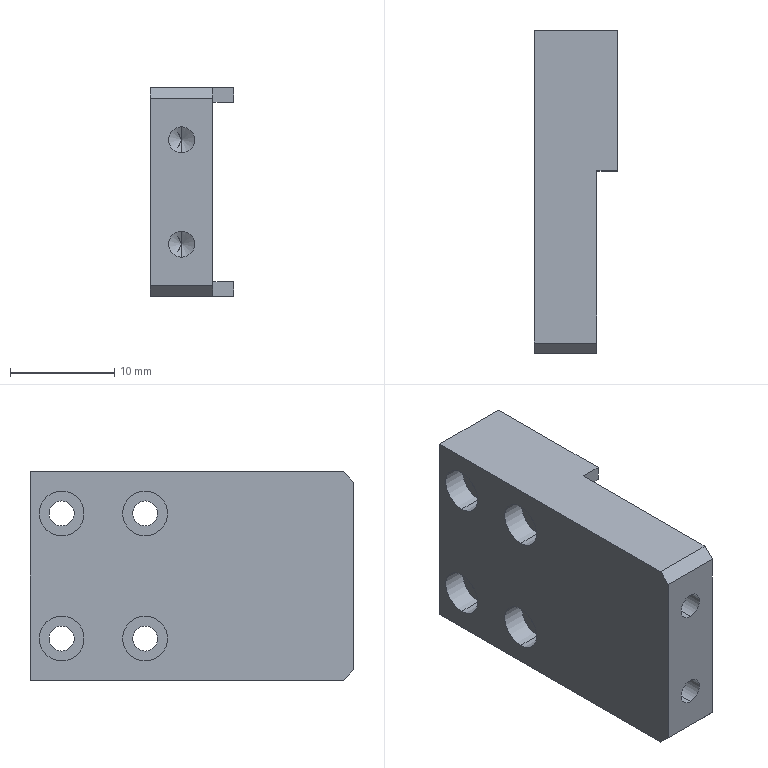Part | SolidWorks | features HoleWzd 2, Chamfer 1, Cut 1, Extrusion 1, ICE 1 | 1 solid | 42 faces | box 8 x 31 x 20 mm | volume 3513 mm3 | cylinder 20 | plane 18 | cone 4 | commonest cylinder face diameters 2.4 x8 4.3 x8 2.5 x4
STEP:
#1=CARTESIAN_POINT('',(3.,-8.,-3.75));
#2=VERTEX_POINT('',#1);
#3=CARTESIAN_POINT('',(3.,-8.,-6.25));
#4=VERTEX_POINT('',#3);
#5=CARTESIAN_POINT('',(3.,-8.,-5.));
#6=DIRECTION('',(0.,-1.,0.));
#7=DIRECTION('',(0.,0.,-1.));
#8=AXIS2_PLACEMENT_3D('',#5,#6,#7);
#9=CIRCLE('',#8,1.25);
#10=EDGE_CURVE('',#2,#4,#9,.T.);
#11=ORIENTED_EDGE('',*,*,#10,.F.);
#12=CARTESIAN_POINT('',(3.,-15.5,-3.75));
#13=VERTEX_POINT('',#12);
#14=CARTESIAN_POINT('',(3.,-15.5,-3.75));
#15=DIRECTION('',(0.,-1.,0.));
#16=VECTOR('',#15,1000.);
#17=LINE('',#14,#16);
#18=EDGE_CURVE('',#2,#13,#17,.T.);
#19=ORIENTED_EDGE('',*,*,#18,.T.);
#20=CARTESIAN_POINT('',(3.,-15.5,-6.25));
#21=VERTEX_POINT('',#20);
#22=CARTESIAN_POINT('',(3.,-15.5,-5.));
#23=DIRECTION('',(0.,-1.,0.));
#24=DIRECTION('',(0.,0.,-1.));
#25=AXIS2_PLACEMENT_3D('',#22,#23,#24);
#26=CIRCLE('',#25,1.25);
#27=EDGE_CURVE('',#13,#21,#26,.T.);
#28=ORIENTED_EDGE('',*,*,#27,.T.);
#29=CARTESIAN_POINT('',(3.,-15.5,-6.25));
#30=DIRECTION('',(0.,-1.,0.));
#31=VECTOR('',#30,1000.);
#32=LINE('',#29,#31);
#33=EDGE_CURVE('',#4,#21,#32,.T.);
#34=ORIENTED_EDGE('',*,*,#33,.F.);
#35=EDGE_LOOP('',(#11,#19,#28,#34));
#36=FACE_OUTER_BOUND('',#35,.T.);
#37=CARTESIAN_POINT('',(3.,-15.5,-5.));
#38=DIRECTION('',(0.,-1.,0.));
#39=DIRECTION('',(0.,0.,-1.));
#40=AXIS2_PLACEMENT_3D('',#37,#38,#39);
#41=CYLINDRICAL_SURFACE('',#40,1.25);
#42=ADVANCED_FACE('',(#36),#41,.F.);
#43=CARTESIAN_POINT('',(3.,-7.249,-5.));
#44=VERTEX_POINT('',#43);
#45=CARTESIAN_POINT('',(3.,-8.,-6.25));
#46=DIRECTION('',(0.,-0.515,-0.8572));
#47=VECTOR('',#46,1000.);
#48=LINE('',#45,#47);
#49=EDGE_CURVE('',#44,#4,#48,.T.);
#50=ORIENTED_EDGE('',*,*,#49,.F.);
#51=CARTESIAN_POINT('',(3.,-8.,-3.75));
#52=DIRECTION('',(0.,-0.515,0.8572));
#53=VECTOR('',#52,1000.);
#54=LINE('',#51,#53);
#55=EDGE_CURVE('',#44,#2,#54,.T.);
#56=ORIENTED_EDGE('',*,*,#55,.T.);
#57=ORIENTED_EDGE('',*,*,#10,.T.);
#58=EDGE_LOOP('',(#50,#56,#57));
#59=FACE_OUTER_BOUND('',#58,.T.);
#60=CARTESIAN_POINT('',(3.,-8.,-5.));
#61=DIRECTION('',(0.,-1.,0.));
#62=DIRECTION('',(0.,0.,-1.));
#63=AXIS2_PLACEMENT_3D('',#60,#61,#62);
#64=CONICAL_SURFACE('',#63,1.25,1.03);
#65=ADVANCED_FACE('',(#59),#64,.F.);
#66=CARTESIAN_POINT('',(3.,-8.,6.25));
#67=VERTEX_POINT('',#66);
#68=CARTESIAN_POINT('',(3.,-8.,3.75));
#69=VERTEX_POINT('',#68);
#70=CARTESIAN_POINT('',(3.,-8.,5.));
#71=DIRECTION('',(0.,-1.,0.));
#72=DIRECTION('',(0.,0.,-1.));
#73=AXIS2_PLACEMENT_3D('',#70,#71,#72);
#74=CIRCLE('',#73,1.25);
#75=EDGE_CURVE('',#67,#69,#74,.T.);
#76=ORIENTED_EDGE('',*,*,#75,.F.);
#77=CARTESIAN_POINT('',(3.,-15.5,6.25));
#78=VERTEX_POINT('',#77);
#79=CARTESIAN_POINT('',(3.,-15.5,6.25));
#80=DIRECTION('',(0.,-1.,0.));
#81=VECTOR('',#80,1000.);
#82=LINE('',#79,#81);
#83=EDGE_CURVE('',#67,#78,#82,.T.);
#84=ORIENTED_EDGE('',*,*,#83,.T.);
#85=CARTESIAN_POINT('',(3.,-15.5,3.75));
#86=VERTEX_POINT('',#85);
#87=CARTESIAN_POINT('',(3.,-15.5,5.));
#88=DIRECTION('',(0.,-1.,0.));
#89=DIRECTION('',(0.,0.,-1.));
#90=AXIS2_PLACEMENT_3D('',#87,#88,#89);
#91=CIRCLE('',#90,1.25);
#92=EDGE_CURVE('',#78,#86,#91,.T.);
#93=ORIENTED_EDGE('',*,*,#92,.T.);
#94=CARTESIAN_POINT('',(3.,-15.5,3.75));
#95=DIRECTION('',(0.,-1.,0.));
#96=VECTOR('',#95,1000.);
#97=LINE('',#94,#96);
#98=EDGE_CURVE('',#69,#86,#97,.T.);
#99=ORIENTED_EDGE('',*,*,#98,.F.);
#100=EDGE_LOOP('',(#76,#84,#93,#99));
#101=FACE_OUTER_BOUND('',#100,.T.);
#102=CARTESIAN_POINT('',(3.,-15.5,5.));
#103=DIRECTION('',(0.,-1.,0.));
#104=DIRECTION('',(0.,0.,-1.));
#105=AXIS2_PLACEMENT_3D('',#102,#103,#104);
#106=CYLINDRICAL_SURFACE('',#105,1.25);
#107=ADVANCED_FACE('',(#101),#106,.F.);
#108=CARTESIAN_POINT('',(3.,-7.249,5.));
#109=VERTEX_POINT('',#108);
#110=CARTESIAN_POINT('',(3.,-8.,3.75));
#111=DIRECTION('',(0.,-0.515,-0.8572));
#112=VECTOR('',#111,1000.);
#113=LINE('',#110,#112);
#114=EDGE_CURVE('',#109,#69,#113,.T.);
#115=ORIENTED_EDGE('',*,*,#114,.F.);
#116=CARTESIAN_POINT('',(3.,-8.,6.25));
#117=DIRECTION('',(0.,-0.515,0.8572));
#118=VECTOR('',#117,1000.);
#119=LINE('',#116,#118);
#120=EDGE_CURVE('',#109,#67,#119,.T.);
#121=ORIENTED_EDGE('',*,*,#120,.T.);
#122=ORIENTED_EDGE('',*,*,#75,.T.);
#123=EDGE_LOOP('',(#115,#121,#122));
#124=FACE_OUTER_BOUND('',#123,.T.);
#125=CARTESIAN_POINT('',(3.,-8.,5.));
#126=DIRECTION('',(0.,-1.,0.));
#127=DIRECTION('',(0.,0.,-1.));
#128=AXIS2_PLACEMENT_3D('',#125,#126,#127);
#129=CONICAL_SURFACE('',#128,1.25,1.03);
#130=ADVANCED_FACE('',(#124),#129,.F.);
#131=CARTESIAN_POINT('',(2.3,12.5,3.85));
#132=VERTEX_POINT('',#131);
#133=CARTESIAN_POINT('',(2.3,12.5,8.15));
#134=VERTEX_POINT('',#133);
#135=CARTESIAN_POINT('',(2.3,12.5,6.));
#136=DIRECTION('',(-1.,0.,0.));
#137=DIRECTION('',(0.,0.,1.));
#138=AXIS2_PLACEMENT_3D('',#135,#136,#137);
#139=CIRCLE('',#138,2.15);
#140=EDGE_CURVE('',#132,#134,#139,.T.);
#141=ORIENTED_EDGE('',*,*,#140,.F.);
#142=CARTESIAN_POINT('',(0.,12.5,3.85));
#143=VERTEX_POINT('',#142);
#144=CARTESIAN_POINT('',(0.,12.5,3.85));
#145=DIRECTION('',(-1.,0.,0.));
#146=VECTOR('',#145,1000.);
#147=LINE('',#144,#146);
#148=EDGE_CURVE('',#132,#143,#147,.T.);
#149=ORIENTED_EDGE('',*,*,#148,.T.);
#150=CARTESIAN_POINT('',(0.,12.5,8.15));
#151=VERTEX_POINT('',#150);
#152=CARTESIAN_POINT('',(0.,12.5,6.));
#153=DIRECTION('',(-1.,0.,0.));
#154=DIRECTION('',(0.,0.,1.));
#155=AXIS2_PLACEMENT_3D('',#152,#153,#154);
#156=CIRCLE('',#155,2.15);
#157=EDGE_CURVE('',#143,#151,#156,.T.);
#158=ORIENTED_EDGE('',*,*,#157,.T.);
#159=CARTESIAN_POINT('',(0.,12.5,8.15));
#160=DIRECTION('',(-1.,0.,0.));
#161=VECTOR('',#160,1000.);
#162=LINE('',#159,#161);
#163=EDGE_CURVE('',#134,#151,#162,.T.);
#164=ORIENTED_EDGE('',*,*,#163,.F.);
#165=EDGE_LOOP('',(#141,#149,#158,#164));
#166=FACE_OUTER_BOUND('',#165,.T.);
#167=CARTESIAN_POINT('',(0.,12.5,6.));
#168=DIRECTION('',(-1.,0.,0.));
#169=DIRECTION('',(0.,0.,1.));
#170=AXIS2_PLACEMENT_3D('',#167,#168,#169);
#171=CYLINDRICAL_SURFACE('',#170,2.15);
#172=ADVANCED_FACE('',(#166),#171,.F.);
#173=CARTESIAN_POINT('',(6.,12.5,4.8));
#174=VERTEX_POINT('',#173);
#175=CARTESIAN_POINT('',(6.,12.5,7.2));
#176=VERTEX_POINT('',#175);
#177=CARTESIAN_POINT('',(6.,12.5,6.));
#178=DIRECTION('',(-1.,0.,0.));
#179=DIRECTION('',(0.,0.,1.));
#180=AXIS2_PLACEMENT_3D('',#177,#178,#179);
#181=CIRCLE('',#180,1.2);
#182=EDGE_CURVE('',#174,#176,#181,.T.);
#183=ORIENTED_EDGE('',*,*,#182,.F.);
#184=CARTESIAN_POINT('',(2.3,12.5,4.8));
#185=VERTEX_POINT('',#184);
#186=CARTESIAN_POINT('',(0.,12.5,4.8));
#187=DIRECTION('',(-1.,0.,0.));
#188=VECTOR('',#187,1000.);
#189=LINE('',#186,#188);
#190=EDGE_CURVE('',#174,#185,#189,.T.);
#191=ORIENTED_EDGE('',*,*,#190,.T.);
#192=CARTESIAN_POINT('',(2.3,12.5,7.2));
#193=VERTEX_POINT('',#192);
#194=CARTESIAN_POINT('',(2.3,12.5,6.));
#195=DIRECTION('',(-1.,0.,0.));
#196=DIRECTION('',(0.,0.,1.));
#197=AXIS2_PLACEMENT_3D('',#194,#195,#196);
#198=CIRCLE('',#197,1.2);
#199=EDGE_CURVE('',#185,#193,#198,.T.);
#200=ORIENTED_EDGE('',*,*,#199,.T.);
#201=CARTESIAN_POINT('',(0.,12.5,7.2));
#202=DIRECTION('',(-1.,0.,0.));
#203=VECTOR('',#202,1000.);
#204=LINE('',#201,#203);
#205=EDGE_CURVE('',#176,#193,#204,.T.);
#206=ORIENTED_EDGE('',*,*,#205,.F.);
#207=EDGE_LOOP('',(#183,#191,#200,#206));
#208=FACE_OUTER_BOUND('',#207,.T.);
#209=CARTESIAN_POINT('',(0.,12.5,6.));
#210=DIRECTION('',(-1.,0.,0.));
#211=DIRECTION('',(0.,0.,1.));
#212=AXIS2_PLACEMENT_3D('',#209,#210,#211);
#213=CYLINDRICAL_SURFACE('',#212,1.2);
#214=ADVANCED_FACE('',(#208),#213,.F.);
#215=CARTESIAN_POINT('',(2.3,12.5,-8.15));
#216=VERTEX_POINT('',#215);
#217=CARTESIAN_POINT('',(2.3,12.5,-3.85));
#218=VERTEX_POINT('',#217);
#219=CARTESIAN_POINT('',(2.3,12.5,-6.));
#220=DIRECTION('',(-1.,0.,0.));
#221=DIRECTION('',(0.,0.,1.));
#222=AXIS2_PLACEMENT_3D('',#219,#220,#221);
#223=CIRCLE('',#222,2.15);
#224=EDGE_CURVE('',#216,#218,#223,.T.);
#225=ORIENTED_EDGE('',*,*,#224,.F.);
#226=CARTESIAN_POINT('',(0.,12.5,-8.15));
#227=VERTEX_POINT('',#226);
#228=CARTESIAN_POINT('',(0.,12.5,-8.15));
#229=DIRECTION('',(-1.,0.,0.));
#230=VECTOR('',#229,1000.);
#231=LINE('',#228,#230);
#232=EDGE_CURVE('',#216,#227,#231,.T.);
#233=ORIENTED_EDGE('',*,*,#232,.T.);
#234=CARTESIAN_POINT('',(0.,12.5,-3.85));
#235=VERTEX_POINT('',#234);
#236=CARTESIAN_POINT('',(0.,12.5,-6.));
#237=DIRECTION('',(-1.,0.,0.));
#238=DIRECTION('',(0.,0.,1.));
#239=AXIS2_PLACEMENT_3D('',#236,#237,#238);
#240=CIRCLE('',#239,2.15);
#241=EDGE_CURVE('',#227,#235,#240,.T.);
#242=ORIENTED_EDGE('',*,*,#241,.T.);
#243=CARTESIAN_POINT('',(0.,12.5,-3.85));
#244=DIRECTION('',(-1.,0.,0.));
#245=VECTOR('',#244,1000.);
#246=LINE('',#243,#245);
#247=EDGE_CURVE('',#218,#235,#246,.T.);
#248=ORIENTED_EDGE('',*,*,#247,.F.);
#249=EDGE_LOOP('',(#225,#233,#242,#248));
#250=FACE_OUTER_BOUND('',#249,.T.);
#251=CARTESIAN_POINT('',(0.,12.5,-6.));
#252=DIRECTION('',(-1.,0.,0.));
#253=DIRECTION('',(0.,0.,1.));
#254=AXIS2_PLACEMENT_3D('',#251,#252,#253);
#255=CYLINDRICAL_SURFACE('',#254,2.15);
#256=ADVANCED_FACE('',(#250),#255,.F.);
#257=CARTESIAN_POINT('',(6.,12.5,-7.2));
#258=VERTEX_POINT('',#257);
#259=CARTESIAN_POINT('',(6.,12.5,-4.8));
#260=VERTEX_POINT('',#259);
#261=CARTESIAN_POINT('',(6.,12.5,-6.));
#262=DIRECTION('',(-1.,0.,0.));
#263=DIRECTION('',(0.,0.,1.));
#264=AXIS2_PLACEMENT_3D('',#261,#262,#263);
#265=CIRCLE('',#264,1.2);
#266=EDGE_CURVE('',#258,#260,#265,.T.);
#267=ORIENTED_EDGE('',*,*,#266,.F.);
#268=CARTESIAN_POINT('',(2.3,12.5,-7.2));
#269=VERTEX_POINT('',#268);
#270=CARTESIAN_POINT('',(0.,12.5,-7.2));
#271=DIRECTION('',(-1.,0.,0.));
#272=VECTOR('',#271,1000.);
#273=LINE('',#270,#272);
#274=EDGE_CURVE('',#258,#269,#273,.T.);
#275=ORIENTED_EDGE('',*,*,#274,.T.);
#276=CARTESIAN_POINT('',(2.3,12.5,-4.8));
#277=VERTEX_POINT('',#276);
#278=CARTESIAN_POINT('',(2.3,12.5,-6.));
#279=DIRECTION('',(-1.,0.,0.));
#280=DIRECTION('',(0.,0.,1.));
#281=AXIS2_PLACEMENT_3D('',#278,#279,#280);
#282=CIRCLE('',#281,1.2);
#283=EDGE_CURVE('',#269,#277,#282,.T.);
#284=ORIENTED_EDGE('',*,*,#283,.T.);
#285=CARTESIAN_POINT('',(0.,12.5,-4.8));
#286=DIRECTION('',(-1.,0.,0.));
#287=VECTOR('',#286,1000.);
#288=LINE('',#285,#287);
#289=EDGE_CURVE('',#260,#277,#288,.T.);
#290=ORIENTED_EDGE('',*,*,#289,.F.);
#291=EDGE_LOOP('',(#267,#275,#284,#290));
#292=FACE_OUTER_BOUND('',#291,.T.);
#293=CARTESIAN_POINT('',(0.,12.5,-6.));
#294=DIRECTION('',(-1.,0.,0.));
#295=DIRECTION('',(0.,0.,1.));
#296=AXIS2_PLACEMENT_3D('',#293,#294,#295);
#297=CYLINDRICAL_SURFACE('',#296,1.2);
#298=ADVANCED_FACE('',(#292),#297,.F.);
#299=CARTESIAN_POINT('',(2.3,4.5,-8.15));
#300=VERTEX_POINT('',#299);
#301=CARTESIAN_POINT('',(2.3,4.5,-3.85));
#302=VERTEX_POINT('',#301);
#303=CARTESIAN_POINT('',(2.3,4.5,-6.));
#304=DIRECTION('',(-1.,0.,0.));
#305=DIRECTION('',(0.,0.,1.));
#306=AXIS2_PLACEMENT_3D('',#303,#304,#305);
#307=CIRCLE('',#306,2.15);
#308=EDGE_CURVE('',#300,#302,#307,.T.);
#309=ORIENTED_EDGE('',*,*,#308,.F.);
#310=CARTESIAN_POINT('',(0.,4.5,-8.15));
#311=VERTEX_POINT('',#310);
#312=CARTESIAN_POINT('',(0.,4.5,-8.15));
#313=DIRECTION('',(-1.,0.,0.));
#314=VECTOR('',#313,1000.);
#315=LINE('',#312,#314);
#316=EDGE_CURVE('',#300,#311,#315,.T.);
#317=ORIENTED_EDGE('',*,*,#316,.T.);
#318=CARTESIAN_POINT('',(0.,4.5,-3.85));
#319=VERTEX_POINT('',#318);
#320=CARTESIAN_POINT('',(0.,4.5,-6.));
#321=DIRECTION('',(-1.,0.,0.));
#322=DIRECTION('',(0.,0.,1.));
#323=AXIS2_PLACEMENT_3D('',#320,#321,#322);
#324=CIRCLE('',#323,2.15);
#325=EDGE_CURVE('',#311,#319,#324,.T.);
#326=ORIENTED_EDGE('',*,*,#325,.T.);
#327=CARTESIAN_POINT('',(0.,4.5,-3.85));
#328=DIRECTION('',(-1.,0.,0.));
#329=VECTOR('',#328,1000.);
#330=LINE('',#327,#329);
#331=EDGE_CURVE('',#302,#319,#330,.T.);
#332=ORIENTED_EDGE('',*,*,#331,.F.);
#333=EDGE_LOOP('',(#309,#317,#326,#332));
#334=FACE_OUTER_BOUND('',#333,.T.);
#335=CARTESIAN_POINT('',(0.,4.5,-6.));
#336=DIRECTION('',(-1.,0.,0.));
#337=DIRECTION('',(0.,0.,1.));
#338=AXIS2_PLACEMENT_3D('',#335,#336,#337);
#339=CYLINDRICAL_SURFACE('',#338,2.15);
#340=ADVANCED_FACE('',(#334),#339,.F.);
#341=CARTESIAN_POINT('',(6.,4.5,-7.2));
#342=VERTEX_POINT('',#341);
#343=CARTESIAN_POINT('',(6.,4.5,-4.8));
#344=VERTEX_POINT('',#343);
#345=CARTESIAN_POINT('',(6.,4.5,-6.));
#346=DIRECTION('',(-1.,0.,0.));
#347=DIRECTION('',(0.,0.,1.));
#348=AXIS2_PLACEMENT_3D('',#345,#346,#347);
#349=CIRCLE('',#348,1.2);
#350=EDGE_CURVE('',#342,#344,#349,.T.);
#351=ORIENTED_EDGE('',*,*,#350,.F.);
#352=CARTESIAN_POINT('',(2.3,4.5,-7.2));
#353=VERTEX_POINT('',#352);
#354=CARTESIAN_POINT('',(0.,4.5,-7.2));
#355=DIRECTION('',(-1.,0.,0.));
#356=VECTOR('',#355,1000.);
#357=LINE('',#354,#356);
#358=EDGE_CURVE('',#342,#353,#357,.T.);
#359=ORIENTED_EDGE('',*,*,#358,.T.);
#360=CARTESIAN_POINT('',(2.3,4.5,-4.8));
#361=VERTEX_POINT('',#360);
#362=CARTESIAN_POINT('',(2.3,4.5,-6.));
#363=DIRECTION('',(-1.,0.,0.));
#364=DIRECTION('',(0.,0.,1.));
#365=AXIS2_PLACEMENT_3D('',#362,#363,#364);
#366=CIRCLE('',#365,1.2);
#367=EDGE_CURVE('',#353,#361,#366,.T.);
#368=ORIENTED_EDGE('',*,*,#367,.T.);
#369=CARTESIAN_POINT('',(0.,4.5,-4.8));
#370=DIRECTION('',(-1.,0.,0.));
#371=VECTOR('',#370,1000.);
#372=LINE('',#369,#371);
#373=EDGE_CURVE('',#344,#361,#372,.T.);
#374=ORIENTED_EDGE('',*,*,#373,.F.);
#375=EDGE_LOOP('',(#351,#359,#368,#374));
#376=FACE_OUTER_BOUND('',#375,.T.);
#377=CARTESIAN_POINT('',(0.,4.5,-6.));
#378=DIRECTION('',(-1.,0.,0.));
#379=DIRECTION('',(0.,0.,1.));
#380=AXIS2_PLACEMENT_3D('',#377,#378,#379);
#381=CYLINDRICAL_SURFACE('',#380,1.2);
#382=ADVANCED_FACE('',(#376),#381,.F.);
#383=CARTESIAN_POINT('',(2.3,4.5,3.85));
#384=VERTEX_POINT('',#383);
#385=CARTESIAN_POINT('',(2.3,4.5,8.15));
#386=VERTEX_POINT('',#385);
#387=CARTESIAN_POINT('',(2.3,4.5,6.));
#388=DIRECTION('',(-1.,0.,0.));
#389=DIRECTION('',(0.,0.,1.));
#390=AXIS2_PLACEMENT_3D('',#387,#388,#389);
#391=CIRCLE('',#390,2.15);
#392=EDGE_CURVE('',#384,#386,#391,.T.);
#393=ORIENTED_EDGE('',*,*,#392,.F.);
#394=CARTESIAN_POINT('',(0.,4.5,3.85));
#395=VERTEX_POINT('',#394);
#396=CARTESIAN_POINT('',(0.,4.5,3.85));
#397=DIRECTION('',(-1.,0.,0.));
#398=VECTOR('',#397,1000.);
#399=LINE('',#396,#398);
#400=EDGE_CURVE('',#384,#395,#399,.T.);
#401=ORIENTED_EDGE('',*,*,#400,.T.);
#402=CARTESIAN_POINT('',(0.,4.5,8.15));
#403=VERTEX_POINT('',#402);
#404=CARTESIAN_POINT('',(0.,4.5,6.));
#405=DIRECTION('',(-1.,0.,0.));
#406=DIRECTION('',(0.,0.,1.));
#407=AXIS2_PLACEMENT_3D('',#404,#405,#406);
#408=CIRCLE('',#407,2.15);
#409=EDGE_CURVE('',#395,#403,#408,.T.);
#410=ORIENTED_EDGE('',*,*,#409,.T.);
#411=CARTESIAN_POINT('',(0.,4.5,8.15));
#412=DIRECTION('',(-1.,0.,0.));
#413=VECTOR('',#412,1000.);
#414=LINE('',#411,#413);
#415=EDGE_CURVE('',#386,#403,#414,.T.);
#416=ORIENTED_EDGE('',*,*,#415,.F.);
#417=EDGE_LOOP('',(#393,#401,#410,#416));
#418=FACE_OUTER_BOUND('',#417,.T.);
#419=CARTESIAN_POINT('',(0.,4.5,6.));
#420=DIRECTION('',(-1.,0.,0.));
#421=DIRECTION('',(0.,0.,1.));
#422=AXIS2_PLACEMENT_3D('',#419,#420,#421);
#423=CYLINDRICAL_SURFACE('',#422,2.15);
#424=ADVANCED_FACE('',(#418),#423,.F.);
#425=CARTESIAN_POINT('',(6.,4.5,4.8));
#426=VERTEX_POINT('',#425);
#427=CARTESIAN_POINT('',(6.,4.5,7.2));
#428=VERTEX_POINT('',#427);
#429=CARTESIAN_POINT('',(6.,4.5,6.));
#430=DIRECTION('',(-1.,0.,0.));
#431=DIRECTION('',(0.,0.,1.));
#432=AXIS2_PLACEMENT_3D('',#429,#430,#431);
#433=CIRCLE('',#432,1.2);
#434=EDGE_CURVE('',#426,#428,#433,.T.);
#435=ORIENTED_EDGE('',*,*,#434,.F.);
#436=CARTESIAN_POINT('',(2.3,4.5,4.8));
#437=VERTEX_POINT('',#436);
#438=CARTESIAN_POINT('',(0.,4.5,4.8));
#439=DIRECTION('',(-1.,0.,0.));
#440=VECTOR('',#439,1000.);
#441=LINE('',#438,#440);
#442=EDGE_CURVE('',#426,#437,#441,.T.);
#443=ORIENTED_EDGE('',*,*,#442,.T.);
#444=CARTESIAN_POINT('',(2.3,4.5,7.2));
#445=VERTEX_POINT('',#444);
#446=CARTESIAN_POINT('',(2.3,4.5,6.));
#447=DIRECTION('',(-1.,0.,0.));
#448=DIRECTION('',(0.,0.,1.));
#449=AXIS2_PLACEMENT_3D('',#446,#447,#448);
#450=CIRCLE('',#449,1.2);
#451=EDGE_CURVE('',#437,#445,#450,.T.);
#452=ORIENTED_EDGE('',*,*,#451,.T.);
#453=CARTESIAN_POINT('',(0.,4.5,7.2));
#454=DIRECTION('',(-1.,0.,0.));
#455=VECTOR('',#454,1000.);
#456=LINE('',#453,#455);
#457=EDGE_CURVE('',#428,#445,#456,.T.);
#458=ORIENTED_EDGE('',*,*,#457,.F.);
#459=EDGE_LOOP('',(#435,#443,#452,#458));
#460=FACE_OUTER_BOUND('',#459,.T.);
#461=CARTESIAN_POINT('',(0.,4.5,6.));
#462=DIRECTION('',(-1.,0.,0.));
#463=DIRECTION('',(0.,0.,1.));
#464=AXIS2_PLACEMENT_3D('',#461,#462,#463);
#465=CYLINDRICAL_SURFACE('',#464,1.2);
#466=ADVANCED_FACE('',(#460),#465,.F.);
#467=CARTESIAN_POINT('',(6.,12.5,6.));
#468=DIRECTION('',(-1.,0.,0.));
#469=DIRECTION('',(0.,0.,1.));
#470=AXIS2_PLACEMENT_3D('',#467,#468,#469);
#471=CIRCLE('',#470,1.2);
#472=EDGE_CURVE('',#176,#174,#471,.T.);
#473=ORIENTED_EDGE('',*,*,#472,.T.);
#474=ORIENTED_EDGE('',*,*,#182,.T.);
#475=EDGE_LOOP('',(#473,#474));
#476=FACE_BOUND('',#475,.T.);
#477=CARTESIAN_POINT('',(6.,12.5,-6.));
#478=DIRECTION('',(-1.,0.,0.));
#479=DIRECTION('',(0.,0.,1.));
#480=AXIS2_PLACEMENT_3D('',#477,#478,#479);
#481=CIRCLE('',#480,1.2);
#482=EDGE_CURVE('',#260,#258,#481,.T.);
#483=ORIENTED_EDGE('',*,*,#482,.T.);
#484=ORIENTED_EDGE('',*,*,#266,.T.);
#485=EDGE_LOOP('',(#483,#484));
#486=FACE_BOUND('',#485,.T.);
#487=CARTESIAN_POINT('',(6.,4.5,-6.));
#488=DIRECTION('',(-1.,0.,0.));
#489=DIRECTION('',(0.,0.,1.));
#490=AXIS2_PLACEMENT_3D('',#487,#488,#489);
#491=CIRCLE('',#490,1.2);
#492=EDGE_CURVE('',#344,#342,#491,.T.);
#493=ORIENTED_EDGE('',*,*,#492,.T.);
#494=ORIENTED_EDGE('',*,*,#350,.T.);
#495=EDGE_LOOP('',(#493,#494));
#496=FACE_BOUND('',#495,.T.);
#497=CARTESIAN_POINT('',(6.,4.5,6.));
#498=DIRECTION('',(-1.,0.,0.));
#499=DIRECTION('',(0.,0.,1.));
#500=AXIS2_PLACEMENT_3D('',#497,#498,#499);
#501=CIRCLE('',#500,1.2);
#502=EDGE_CURVE('',#428,#426,#501,.T.);
#503=ORIENTED_EDGE('',*,*,#502,.T.);
#504=ORIENTED_EDGE('',*,*,#434,.T.);
#505=EDGE_LOOP('',(#503,#504));
#506=FACE_BOUND('',#505,.T.);
#507=CARTESIAN_POINT('',(6.,2.,10.));
#508=VERTEX_POINT('',#507);
#509=CARTESIAN_POINT('',(6.,-14.5,10.));
#510=VERTEX_POINT('',#509);
#511=CARTESIAN_POINT('',(6.,-15.5,10.));
#512=DIRECTION('',(0.,-1.,0.));
#513=VECTOR('',#512,1000.);
#514=LINE('',#511,#513);
#515=EDGE_CURVE('',#508,#510,#514,.T.);
#516=ORIENTED_EDGE('',*,*,#515,.T.);
#517=CARTESIAN_POINT('',(6.,-15.5,9.));
#518=VERTEX_POINT('',#517);
#519=CARTESIAN_POINT('',(6.,-15.5,9.));
#520=DIRECTION('',(0.,-0.7071,-0.7071));
#521=VECTOR('',#520,1000.);
#522=LINE('',#519,#521);
#523=EDGE_CURVE('',#510,#518,#522,.T.);
#524=ORIENTED_EDGE('',*,*,#523,.T.);
#525=CARTESIAN_POINT('',(6.,-15.5,-9.));
#526=VERTEX_POINT('',#525);
#527=CARTESIAN_POINT('',(6.,-15.5,10.));
#528=DIRECTION('',(0.,0.,-1.));
#529=VECTOR('',#528,1000.);
#530=LINE('',#527,#529);
#531=EDGE_CURVE('',#518,#526,#530,.T.);
#532=ORIENTED_EDGE('',*,*,#531,.T.);
#533=CARTESIAN_POINT('',(6.,-14.5,-10.));
#534=VERTEX_POINT('',#533);
#535=CARTESIAN_POINT('',(6.,-14.5,-10.));
#536=DIRECTION('',(0.,0.7071,-0.7071));
#537=VECTOR('',#536,1000.);
#538=LINE('',#535,#537);
#539=EDGE_CURVE('',#526,#534,#538,.T.);
#540=ORIENTED_EDGE('',*,*,#539,.T.);
#541=CARTESIAN_POINT('',(6.,2.,-10.));
#542=VERTEX_POINT('',#541);
#543=CARTESIAN_POINT('',(6.,-15.5,-10.));
#544=DIRECTION('',(0.,-1.,0.));
#545=VECTOR('',#544,1000.);
#546=LINE('',#543,#545);
#547=EDGE_CURVE('',#542,#534,#546,.T.);
#548=ORIENTED_EDGE('',*,*,#547,.F.);
#549=CARTESIAN_POINT('',(6.,2.,-8.6));
#550=VERTEX_POINT('',#549);
#551=CARTESIAN_POINT('',(6.,2.,-10.));
#552=DIRECTION('',(0.,0.,1.));
#553=VECTOR('',#552,1000.);
#554=LINE('',#551,#553);
#555=EDGE_CURVE('',#542,#550,#554,.T.);
#556=ORIENTED_EDGE('',*,*,#555,.T.);
#557=CARTESIAN_POINT('',(6.,15.5,-8.6));
#558=VERTEX_POINT('',#557);
#559=CARTESIAN_POINT('',(6.,15.5,-8.6));
#560=DIRECTION('',(0.,-1.,0.));
#561=VECTOR('',#560,1000.);
#562=LINE('',#559,#561);
#563=EDGE_CURVE('',#558,#550,#562,.T.);
#564=ORIENTED_EDGE('',*,*,#563,.F.);
#565=CARTESIAN_POINT('',(6.,15.5,8.6));
#566=VERTEX_POINT('',#565);
#567=CARTESIAN_POINT('',(6.,15.5,10.));
#568=DIRECTION('',(0.,0.,1.));
#569=VECTOR('',#568,1000.);
#570=LINE('',#567,#569);
#571=EDGE_CURVE('',#558,#566,#570,.T.);
#572=ORIENTED_EDGE('',*,*,#571,.T.);
#573=CARTESIAN_POINT('',(6.,2.,8.6));
#574=VERTEX_POINT('',#573);
#575=CARTESIAN_POINT('',(6.,15.5,8.6));
#576=DIRECTION('',(0.,1.,0.));
#577=VECTOR('',#576,1000.);
#578=LINE('',#575,#577);
#579=EDGE_CURVE('',#574,#566,#578,.T.);
#580=ORIENTED_EDGE('',*,*,#579,.F.);
#581=CARTESIAN_POINT('',(6.,2.,-10.));
#582=DIRECTION('',(0.,0.,1.));
#583=VECTOR('',#582,1000.);
#584=LINE('',#581,#583);
#585=EDGE_CURVE('',#574,#508,#584,.T.);
#586=ORIENTED_EDGE('',*,*,#585,.T.);
#587=EDGE_LOOP('',(#516,#524,#532,#540,#548,#556,#564,#572,#580,#586));
#588=FACE_OUTER_BOUND('',#587,.T.);
#589=CARTESIAN_POINT('',(6.,0.,0.));
#590=DIRECTION('',(-1.,0.,0.));
#591=DIRECTION('',(0.,0.,1.));
#592=AXIS2_PLACEMENT_3D('',#589,#590,#591);
#593=PLANE('',#592);
#594=ADVANCED_FACE('',(#476,#486,#496,#506,#588),#593,.F.);
#595=ORIENTED_EDGE('',*,*,#547,.T.);
#596=CARTESIAN_POINT('',(0.,-14.5,-10.));
#597=VERTEX_POINT('',#596);
#598=CARTESIAN_POINT('',(6.,-14.5,-10.));
#599=DIRECTION('',(-1.,0.,0.));
#600=VECTOR('',#599,1000.);
#601=LINE('',#598,#600);
#602=EDGE_CURVE('',#534,#597,#601,.T.);
#603=ORIENTED_EDGE('',*,*,#602,.T.);
#604=CARTESIAN_POINT('',(0.,15.5,-10.));
#605=VERTEX_POINT('',#604);
#606=CARTESIAN_POINT('',(0.,-15.5,-10.));
#607=DIRECTION('',(0.,1.,0.));
#608=VECTOR('',#607,1000.);
#609=LINE('',#606,#608);
#610=EDGE_CURVE('',#597,#605,#609,.T.);
#611=ORIENTED_EDGE('',*,*,#610,.T.);
#612=CARTESIAN_POINT('',(8.,15.5,-10.));
#613=VERTEX_POINT('',#612);
#614=CARTESIAN_POINT('',(6.,15.5,-10.));
#615=DIRECTION('',(-1.,0.,0.));
#616=VECTOR('',#615,1000.);
#617=LINE('',#614,#616);
#618=EDGE_CURVE('',#613,#605,#617,.T.);
#619=ORIENTED_EDGE('',*,*,#618,.F.);
#620=CARTESIAN_POINT('',(8.,2.,-10.));
#621=VERTEX_POINT('',#620);
#622=CARTESIAN_POINT('',(8.,15.5,-10.));
#623=DIRECTION('',(0.,1.,0.));
#624=VECTOR('',#623,1000.);
#625=LINE('',#622,#624);
#626=EDGE_CURVE('',#621,#613,#625,.T.);
#627=ORIENTED_EDGE('',*,*,#626,.F.);
#628=CARTESIAN_POINT('',(8.,2.,-10.));
#629=DIRECTION('',(-1.,0.,0.));
#630=VECTOR('',#629,1000.);
#631=LINE('',#628,#630);
#632=EDGE_CURVE('',#621,#542,#631,.T.);
#633=ORIENTED_EDGE('',*,*,#632,.T.);
#634=EDGE_LOOP('',(#595,#603,#611,#619,#627,#633));
#635=FACE_OUTER_BOUND('',#634,.T.);
#636=CARTESIAN_POINT('',(6.,-15.5,-10.));
#637=DIRECTION('',(0.,0.,1.));
#638=DIRECTION('',(1.,0.,0.));
#639=AXIS2_PLACEMENT_3D('',#636,#637,#638);
#640=PLANE('',#639);
#641=ADVANCED_FACE('',(#635),#640,.F.);
#642=CARTESIAN_POINT('',(0.,15.5,10.));
#643=VERTEX_POINT('',#642);
#644=CARTESIAN_POINT('',(0.,15.5,10.));
#645=DIRECTION('',(0.,0.,1.));
#646=VECTOR('',#645,1000.);
#647=LINE('',#644,#646);
#648=EDGE_CURVE('',#605,#643,#647,.T.);
#649=ORIENTED_EDGE('',*,*,#648,.T.);
#650=CARTESIAN_POINT('',(8.,15.5,10.));
#651=VERTEX_POINT('',#650);
#652=CARTESIAN_POINT('',(6.,15.5,10.));
#653=DIRECTION('',(-1.,0.,0.));
#654=VECTOR('',#653,1000.);
#655=LINE('',#652,#654);
#656=EDGE_CURVE('',#651,#643,#655,.T.);
#657=ORIENTED_EDGE('',*,*,#656,.F.);
#658=CARTESIAN_POINT('',(8.,15.5,8.6));
#659=VERTEX_POINT('',#658);
#660=CARTESIAN_POINT('',(8.,15.5,10.));
#661=DIRECTION('',(0.,0.,1.));
#662=VECTOR('',#661,1000.);
#663=LINE('',#660,#662);
#664=EDGE_CURVE('',#659,#651,#663,.T.);
#665=ORIENTED_EDGE('',*,*,#664,.F.);
#666=CARTESIAN_POINT('',(8.,15.5,8.6));
#667=DIRECTION('',(-1.,0.,0.));
#668=VECTOR('',#667,1000.);
#669=LINE('',#666,#668);
#670=EDGE_CURVE('',#659,#566,#669,.T.);
#671=ORIENTED_EDGE('',*,*,#670,.T.);
#672=ORIENTED_EDGE('',*,*,#571,.F.);
#673=CARTESIAN_POINT('',(8.,15.5,-8.6));
#674=VERTEX_POINT('',#673);
#675=CARTESIAN_POINT('',(8.,15.5,-8.6));
#676=DIRECTION('',(-1.,0.,0.));
#677=VECTOR('',#676,1000.);
#678=LINE('',#675,#677);
#679=EDGE_CURVE('',#674,#558,#678,.T.);
#680=ORIENTED_EDGE('',*,*,#679,.F.);
#681=CARTESIAN_POINT('',(8.,15.5,-10.));
#682=DIRECTION('',(0.,0.,1.));
#683=VECTOR('',#682,1000.);
#684=LINE('',#681,#683);
#685=EDGE_CURVE('',#613,#674,#684,.T.);
#686=ORIENTED_EDGE('',*,*,#685,.F.);
#687=ORIENTED_EDGE('',*,*,#618,.T.);
#688=EDGE_LOOP('',(#649,#657,#665,#671,#672,#680,#686,#687));
#689=FACE_OUTER_BOUND('',#688,.T.);
#690=CARTESIAN_POINT('',(6.,15.5,10.));
#691=DIRECTION('',(0.,-1.,0.));
#692=DIRECTION('',(0.,0.,-1.));
#693=AXIS2_PLACEMENT_3D('',#690,#691,#692);
#694=PLANE('',#693);
#695=ADVANCED_FACE('',(#689),#694,.F.);
#696=CARTESIAN_POINT('',(0.,-14.5,10.));
#697=VERTEX_POINT('',#696);
#698=CARTESIAN_POINT('',(0.,-15.5,10.));
#699=DIRECTION('',(0.,-1.,0.));
#700=VECTOR('',#699,1000.);
#701=LINE('',#698,#700);
#702=EDGE_CURVE('',#643,#697,#701,.T.);
#703=ORIENTED_EDGE('',*,*,#702,.T.);
#704=CARTESIAN_POINT('',(6.,-14.5,10.));
#705=DIRECTION('',(1.,0.,0.));
#706=VECTOR('',#705,1000.);
#707=LINE('',#704,#706);
#708=EDGE_CURVE('',#697,#510,#707,.T.);
#709=ORIENTED_EDGE('',*,*,#708,.T.);
#710=ORIENTED_EDGE('',*,*,#515,.F.);
#711=CARTESIAN_POINT('',(8.,2.,10.));
#712=VERTEX_POINT('',#711);
#713=CARTESIAN_POINT('',(8.,2.,10.));
#714=DIRECTION('',(-1.,0.,0.));
#715=VECTOR('',#714,1000.);
#716=LINE('',#713,#715);
#717=EDGE_CURVE('',#712,#508,#716,.T.);
#718=ORIENTED_EDGE('',*,*,#717,.F.);
#719=CARTESIAN_POINT('',(8.,15.5,10.));
#720=DIRECTION('',(0.,-1.,0.));
#721=VECTOR('',#720,1000.);
#722=LINE('',#719,#721);
#723=EDGE_CURVE('',#651,#712,#722,.T.);
#724=ORIENTED_EDGE('',*,*,#723,.F.);
#725=ORIENTED_EDGE('',*,*,#656,.T.);
#726=EDGE_LOOP('',(#703,#709,#710,#718,#724,#725));
#727=FACE_OUTER_BOUND('',#726,.T.);
#728=CARTESIAN_POINT('',(6.,-15.5,10.));
#729=DIRECTION('',(0.,0.,-1.));
#730=DIRECTION('',(-1.,0.,0.));
#731=AXIS2_PLACEMENT_3D('',#728,#729,#730);
#732=PLANE('',#731);
#733=ADVANCED_FACE('',(#727),#732,.F.);
#734=CARTESIAN_POINT('',(3.,-15.5,-5.));
#735=DIRECTION('',(0.,-1.,0.));
#736=DIRECTION('',(0.,0.,-1.));
#737=AXIS2_PLACEMENT_3D('',#734,#735,#736);
#738=CIRCLE('',#737,1.25);
#739=EDGE_CURVE('',#21,#13,#738,.T.);
#740=ORIENTED_EDGE('',*,*,#739,.F.);
#741=ORIENTED_EDGE('',*,*,#27,.F.);
#742=EDGE_LOOP('',(#740,#741));
#743=FACE_BOUND('',#742,.T.);
#744=CARTESIAN_POINT('',(3.,-15.5,5.));
#745=DIRECTION('',(0.,-1.,0.));
#746=DIRECTION('',(0.,0.,-1.));
#747=AXIS2_PLACEMENT_3D('',#744,#745,#746);
#748=CIRCLE('',#747,1.25);
#749=EDGE_CURVE('',#86,#78,#748,.T.);
#750=ORIENTED_EDGE('',*,*,#749,.F.);
#751=ORIENTED_EDGE('',*,*,#92,.F.);
#752=EDGE_LOOP('',(#750,#751));
#753=FACE_BOUND('',#752,.T.);
#754=ORIENTED_EDGE('',*,*,#531,.F.);
#755=CARTESIAN_POINT('',(0.,-15.5,9.));
#756=VERTEX_POINT('',#755);
#757=CARTESIAN_POINT('',(6.,-15.5,9.));
#758=DIRECTION('',(-1.,0.,0.));
#759=VECTOR('',#758,1000.);
#760=LINE('',#757,#759);
#761=EDGE_CURVE('',#518,#756,#760,.T.);
#762=ORIENTED_EDGE('',*,*,#761,.T.);
#763=CARTESIAN_POINT('',(0.,-15.5,-9.));
#764=VERTEX_POINT('',#763);
#765=CARTESIAN_POINT('',(0.,-15.5,10.));
#766=DIRECTION('',(0.,0.,-1.));
#767=VECTOR('',#766,1000.);
#768=LINE('',#765,#767);
#769=EDGE_CURVE('',#756,#764,#768,.T.);
#770=ORIENTED_EDGE('',*,*,#769,.T.);
#771=CARTESIAN_POINT('',(6.,-15.5,-9.));
#772=DIRECTION('',(1.,0.,0.));
#773=VECTOR('',#772,1000.);
#774=LINE('',#771,#773);
#775=EDGE_CURVE('',#764,#526,#774,.T.);
#776=ORIENTED_EDGE('',*,*,#775,.T.);
#777=EDGE_LOOP('',(#754,#762,#770,#776));
#778=FACE_OUTER_BOUND('',#777,.T.);
#779=CARTESIAN_POINT('',(6.,-15.5,10.));
#780=DIRECTION('',(0.,1.,0.));
#781=DIRECTION('',(0.,0.,1.));
#782=AXIS2_PLACEMENT_3D('',#779,#780,#781);
#783=PLANE('',#782);
#784=ADVANCED_FACE('',(#743,#753,#778),#783,.F.);
#785=CARTESIAN_POINT('',(0.,12.5,6.));
#786=DIRECTION('',(-1.,0.,0.));
#787=DIRECTION('',(0.,0.,1.));
#788=AXIS2_PLACEMENT_3D('',#785,#786,#787);
#789=CIRCLE('',#788,2.15);
#790=EDGE_CURVE('',#151,#143,#789,.T.);
#791=ORIENTED_EDGE('',*,*,#790,.F.);
#792=ORIENTED_EDGE('',*,*,#157,.F.);
#793=EDGE_LOOP('',(#791,#792));
#794=FACE_BOUND('',#793,.T.);
#795=CARTESIAN_POINT('',(0.,12.5,-6.));
#796=DIRECTION('',(-1.,0.,0.));
#797=DIRECTION('',(0.,0.,1.));
#798=AXIS2_PLACEMENT_3D('',#795,#796,#797);
#799=CIRCLE('',#798,2.15);
#800=EDGE_CURVE('',#235,#227,#799,.T.);
#801=ORIENTED_EDGE('',*,*,#800,.F.);
#802=ORIENTED_EDGE('',*,*,#241,.F.);
#803=EDGE_LOOP('',(#801,#802));
#804=FACE_BOUND('',#803,.T.);
#805=CARTESIAN_POINT('',(0.,4.5,-6.));
#806=DIRECTION('',(-1.,0.,0.));
#807=DIRECTION('',(0.,0.,1.));
#808=AXIS2_PLACEMENT_3D('',#805,#806,#807);
#809=CIRCLE('',#808,2.15);
#810=EDGE_CURVE('',#319,#311,#809,.T.);
#811=ORIENTED_EDGE('',*,*,#810,.F.);
#812=ORIENTED_EDGE('',*,*,#325,.F.);
#813=EDGE_LOOP('',(#811,#812));
#814=FACE_BOUND('',#813,.T.);
#815=CARTESIAN_POINT('',(0.,4.5,6.));
#816=DIRECTION('',(-1.,0.,0.));
#817=DIRECTION('',(0.,0.,1.));
#818=AXIS2_PLACEMENT_3D('',#815,#816,#817);
#819=CIRCLE('',#818,2.15);
#820=EDGE_CURVE('',#403,#395,#819,.T.);
#821=ORIENTED_EDGE('',*,*,#820,.F.);
#822=ORIENTED_EDGE('',*,*,#409,.F.);
#823=EDGE_LOOP('',(#821,#822));
#824=FACE_BOUND('',#823,.T.);
#825=ORIENTED_EDGE('',*,*,#769,.F.);
#826=CARTESIAN_POINT('',(0.,-12.25,12.25));
#827=DIRECTION('',(0.,0.7071,0.7071));
#828=VECTOR('',#827,1000.);
#829=LINE('',#826,#828);
#830=EDGE_CURVE('',#756,#697,#829,.T.);
#831=ORIENTED_EDGE('',*,*,#830,.T.);
#832=ORIENTED_EDGE('',*,*,#702,.F.);
#833=ORIENTED_EDGE('',*,*,#648,.F.);
#834=ORIENTED_EDGE('',*,*,#610,.F.);
#835=CARTESIAN_POINT('',(0.,-12.25,-12.25));
#836=DIRECTION('',(0.,-0.7071,0.7071));
#837=VECTOR('',#836,1000.);
#838=LINE('',#835,#837);
#839=EDGE_CURVE('',#597,#764,#838,.T.);
#840=ORIENTED_EDGE('',*,*,#839,.T.);
#841=EDGE_LOOP('',(#825,#831,#832,#833,#834,#840));
#842=FACE_OUTER_BOUND('',#841,.T.);
#843=CARTESIAN_POINT('',(0.,0.,0.));
#844=DIRECTION('',(-1.,0.,0.));
#845=DIRECTION('',(0.,0.,1.));
#846=AXIS2_PLACEMENT_3D('',#843,#844,#845);
#847=PLANE('',#846);
#848=ADVANCED_FACE('',(#794,#804,#814,#824,#842),#847,.T.);
#849=CARTESIAN_POINT('',(8.,2.,8.6));
#850=VERTEX_POINT('',#849);
#851=CARTESIAN_POINT('',(8.,15.5,8.6));
#852=DIRECTION('',(0.,1.,0.));
#853=VECTOR('',#852,1000.);
#854=LINE('',#851,#853);
#855=EDGE_CURVE('',#850,#659,#854,.T.);
#856=ORIENTED_EDGE('',*,*,#855,.F.);
#857=CARTESIAN_POINT('',(8.,2.,8.6));
#858=DIRECTION('',(-1.,0.,0.));
#859=VECTOR('',#858,1000.);
#860=LINE('',#857,#859);
#861=EDGE_CURVE('',#850,#574,#860,.T.);
#862=ORIENTED_EDGE('',*,*,#861,.T.);
#863=ORIENTED_EDGE('',*,*,#579,.T.);
#864=ORIENTED_EDGE('',*,*,#670,.F.);
#865=EDGE_LOOP('',(#856,#862,#863,#864));
#866=FACE_OUTER_BOUND('',#865,.T.);
#867=CARTESIAN_POINT('',(8.,15.5,8.6));
#868=DIRECTION('',(0.,0.,1.));
#869=DIRECTION('',(0.,-1.,0.));
#870=AXIS2_PLACEMENT_3D('',#867,#868,#869);
#871=PLANE('',#870);
#872=ADVANCED_FACE('',(#866),#871,.F.);
#873=CARTESIAN_POINT('',(8.,2.,-10.));
#874=DIRECTION('',(0.,0.,1.));
#875=VECTOR('',#874,1000.);
#876=LINE('',#873,#875);
#877=EDGE_CURVE('',#850,#712,#876,.T.);
#878=ORIENTED_EDGE('',*,*,#877,.F.);
#879=ORIENTED_EDGE('',*,*,#855,.T.);
#880=ORIENTED_EDGE('',*,*,#664,.T.);
#881=ORIENTED_EDGE('',*,*,#723,.T.);
#882=EDGE_LOOP('',(#878,#879,#880,#881));
#883=FACE_OUTER_BOUND('',#882,.T.);
#884=CARTESIAN_POINT('',(8.,0.,0.));
#885=DIRECTION('',(1.,0.,0.));
#886=DIRECTION('',(0.,0.,-1.));
#887=AXIS2_PLACEMENT_3D('',#884,#885,#886);
#888=PLANE('',#887);
#889=ADVANCED_FACE('',(#883),#888,.T.);
#890=ORIENTED_EDGE('',*,*,#563,.T.);
#891=CARTESIAN_POINT('',(8.,2.,-8.6));
#892=VERTEX_POINT('',#891);
#893=CARTESIAN_POINT('',(8.,2.,-8.6));
#894=DIRECTION('',(1.,0.,0.));
#895=VECTOR('',#894,1000.);
#896=LINE('',#893,#895);
#897=EDGE_CURVE('',#550,#892,#896,.T.);
#898=ORIENTED_EDGE('',*,*,#897,.T.);
#899=CARTESIAN_POINT('',(8.,15.5,-8.6));
#900=DIRECTION('',(0.,-1.,0.));
#901=VECTOR('',#900,1000.);
#902=LINE('',#899,#901);
#903=EDGE_CURVE('',#674,#892,#902,.T.);
#904=ORIENTED_EDGE('',*,*,#903,.F.);
#905=ORIENTED_EDGE('',*,*,#679,.T.);
#906=EDGE_LOOP('',(#890,#898,#904,#905));
#907=FACE_OUTER_BOUND('',#906,.T.);
#908=CARTESIAN_POINT('',(8.,15.5,-8.6));
#909=DIRECTION('',(0.,0.,-1.));
#910=DIRECTION('',(0.,1.,0.));
#911=AXIS2_PLACEMENT_3D('',#908,#909,#910);
#912=PLANE('',#911);
#913=ADVANCED_FACE('',(#907),#912,.F.);
#914=CARTESIAN_POINT('',(8.,2.,-10.));
#915=DIRECTION('',(0.,0.,1.));
#916=VECTOR('',#915,1000.);
#917=LINE('',#914,#916);
#918=EDGE_CURVE('',#621,#892,#917,.T.);
#919=ORIENTED_EDGE('',*,*,#918,.F.);
#920=ORIENTED_EDGE('',*,*,#626,.T.);
#921=ORIENTED_EDGE('',*,*,#685,.T.);
#922=ORIENTED_EDGE('',*,*,#903,.T.);
#923=EDGE_LOOP('',(#919,#920,#921,#922));
#924=FACE_OUTER_BOUND('',#923,.T.);
#925=CARTESIAN_POINT('',(8.,0.,0.));
#926=DIRECTION('',(1.,0.,0.));
#927=DIRECTION('',(0.,0.,-1.));
#928=AXIS2_PLACEMENT_3D('',#925,#926,#927);
#929=PLANE('',#928);
#930=ADVANCED_FACE('',(#924),#929,.T.);
#931=ORIENTED_EDGE('',*,*,#555,.F.);
#932=ORIENTED_EDGE('',*,*,#632,.F.);
#933=ORIENTED_EDGE('',*,*,#918,.T.);
#934=ORIENTED_EDGE('',*,*,#897,.F.);
#935=EDGE_LOOP('',(#931,#932,#933,#934));
#936=FACE_OUTER_BOUND('',#935,.T.);
#937=CARTESIAN_POINT('',(8.,2.,-10.));
#938=DIRECTION('',(0.,1.,0.));
#939=DIRECTION('',(0.,0.,1.));
#940=AXIS2_PLACEMENT_3D('',#937,#938,#939);
#941=PLANE('',#940);
#942=ADVANCED_FACE('',(#936),#941,.F.);
#943=ORIENTED_EDGE('',*,*,#877,.T.);
#944=ORIENTED_EDGE('',*,*,#717,.T.);
#945=ORIENTED_EDGE('',*,*,#585,.F.);
#946=ORIENTED_EDGE('',*,*,#861,.F.);
#947=EDGE_LOOP('',(#943,#944,#945,#946));
#948=FACE_OUTER_BOUND('',#947,.T.);
#949=CARTESIAN_POINT('',(8.,2.,-10.));
#950=DIRECTION('',(0.,1.,0.));
#951=DIRECTION('',(0.,0.,1.));
#952=AXIS2_PLACEMENT_3D('',#949,#950,#951);
#953=PLANE('',#952);
#954=ADVANCED_FACE('',(#948),#953,.F.);
#955=ORIENTED_EDGE('',*,*,#442,.F.);
#956=ORIENTED_EDGE('',*,*,#502,.F.);
#957=ORIENTED_EDGE('',*,*,#457,.T.);
#958=CARTESIAN_POINT('',(2.3,4.5,6.));
#959=DIRECTION('',(-1.,0.,0.));
#960=DIRECTION('',(0.,0.,1.));
#961=AXIS2_PLACEMENT_3D('',#958,#959,#960);
#962=CIRCLE('',#961,1.2);
#963=EDGE_CURVE('',#445,#437,#962,.T.);
#964=ORIENTED_EDGE('',*,*,#963,.T.);
#965=EDGE_LOOP('',(#955,#956,#957,#964));
#966=FACE_OUTER_BOUND('',#965,.T.);
#967=CARTESIAN_POINT('',(0.,4.5,6.));
#968=DIRECTION('',(-1.,0.,0.));
#969=DIRECTION('',(0.,0.,1.));
#970=AXIS2_PLACEMENT_3D('',#967,#968,#969);
#971=CYLINDRICAL_SURFACE('',#970,1.2);
#972=ADVANCED_FACE('',(#966),#971,.F.);
#973=ORIENTED_EDGE('',*,*,#963,.F.);
#974=ORIENTED_EDGE('',*,*,#451,.F.);
#975=EDGE_LOOP('',(#973,#974));
#976=FACE_BOUND('',#975,.T.);
#977=CARTESIAN_POINT('',(2.3,4.5,6.));
#978=DIRECTION('',(-1.,0.,0.));
#979=DIRECTION('',(0.,0.,1.));
#980=AXIS2_PLACEMENT_3D('',#977,#978,#979);
#981=CIRCLE('',#980,2.15);
#982=EDGE_CURVE('',#386,#384,#981,.T.);
#983=ORIENTED_EDGE('',*,*,#982,.T.);
#984=ORIENTED_EDGE('',*,*,#392,.T.);
#985=EDGE_LOOP('',(#983,#984));
#986=FACE_OUTER_BOUND('',#985,.T.);
#987=CARTESIAN_POINT('',(2.3,5.7,6.));
#988=DIRECTION('',(1.,0.,0.));
#989=DIRECTION('',(0.,0.,-1.));
#990=AXIS2_PLACEMENT_3D('',#987,#988,#989);
#991=PLANE('',#990);
#992=ADVANCED_FACE('',(#976,#986),#991,.F.);
#993=ORIENTED_EDGE('',*,*,#400,.F.);
#994=ORIENTED_EDGE('',*,*,#982,.F.);
#995=ORIENTED_EDGE('',*,*,#415,.T.);
#996=ORIENTED_EDGE('',*,*,#820,.T.);
#997=EDGE_LOOP('',(#993,#994,#995,#996));
#998=FACE_OUTER_BOUND('',#997,.T.);
#999=CARTESIAN_POINT('',(0.,4.5,6.));
#1000=DIRECTION('',(-1.,0.,0.));
#1001=DIRECTION('',(0.,0.,1.));
#1002=AXIS2_PLACEMENT_3D('',#999,#1000,#1001);
#1003=CYLINDRICAL_SURFACE('',#1002,2.15);
#1004=ADVANCED_FACE('',(#998),#1003,.F.);
#1005=ORIENTED_EDGE('',*,*,#358,.F.);
#1006=ORIENTED_EDGE('',*,*,#492,.F.);
#1007=ORIENTED_EDGE('',*,*,#373,.T.);
#1008=CARTESIAN_POINT('',(2.3,4.5,-6.));
#1009=DIRECTION('',(-1.,0.,0.));
#1010=DIRECTION('',(0.,0.,1.));
#1011=AXIS2_PLACEMENT_3D('',#1008,#1009,#1010);
#1012=CIRCLE('',#1011,1.2);
#1013=EDGE_CURVE('',#361,#353,#1012,.T.);
#1014=ORIENTED_EDGE('',*,*,#1013,.T.);
#1015=EDGE_LOOP('',(#1005,#1006,#1007,#1014));
#1016=FACE_OUTER_BOUND('',#1015,.T.);
#1017=CARTESIAN_POINT('',(0.,4.5,-6.));
#1018=DIRECTION('',(-1.,0.,0.));
#1019=DIRECTION('',(0.,0.,1.));
#1020=AXIS2_PLACEMENT_3D('',#1017,#1018,#1019);
#1021=CYLINDRICAL_SURFACE('',#1020,1.2);
#1022=ADVANCED_FACE('',(#1016),#1021,.F.);
#1023=ORIENTED_EDGE('',*,*,#1013,.F.);
#1024=ORIENTED_EDGE('',*,*,#367,.F.);
#1025=EDGE_LOOP('',(#1023,#1024));
#1026=FACE_BOUND('',#1025,.T.);
#1027=CARTESIAN_POINT('',(2.3,4.5,-6.));
#1028=DIRECTION('',(-1.,0.,0.));
#1029=DIRECTION('',(0.,0.,1.));
#1030=AXIS2_PLACEMENT_3D('',#1027,#1028,#1029);
#1031=CIRCLE('',#1030,2.15);
#1032=EDGE_CURVE('',#302,#300,#1031,.T.);
#1033=ORIENTED_EDGE('',*,*,#1032,.T.);
#1034=ORIENTED_EDGE('',*,*,#308,.T.);
#1035=EDGE_LOOP('',(#1033,#1034));
#1036=FACE_OUTER_BOUND('',#1035,.T.);
#1037=CARTESIAN_POINT('',(2.3,5.7,-6.));
#1038=DIRECTION('',(1.,0.,0.));
#1039=DIRECTION('',(0.,0.,-1.));
#1040=AXIS2_PLACEMENT_3D('',#1037,#1038,#1039);
#1041=PLANE('',#1040);
#1042=ADVANCED_FACE('',(#1026,#1036),#1041,.F.);
#1043=ORIENTED_EDGE('',*,*,#316,.F.);
#1044=ORIENTED_EDGE('',*,*,#1032,.F.);
#1045=ORIENTED_EDGE('',*,*,#331,.T.);
#1046=ORIENTED_EDGE('',*,*,#810,.T.);
#1047=EDGE_LOOP('',(#1043,#1044,#1045,#1046));
#1048=FACE_OUTER_BOUND('',#1047,.T.);
#1049=CARTESIAN_POINT('',(0.,4.5,-6.));
#1050=DIRECTION('',(-1.,0.,0.));
#1051=DIRECTION('',(0.,0.,1.));
#1052=AXIS2_PLACEMENT_3D('',#1049,#1050,#1051);
#1053=CYLINDRICAL_SURFACE('',#1052,2.15);
#1054=ADVANCED_FACE('',(#1048),#1053,.F.);
#1055=ORIENTED_EDGE('',*,*,#274,.F.);
#1056=ORIENTED_EDGE('',*,*,#482,.F.);
#1057=ORIENTED_EDGE('',*,*,#289,.T.);
#1058=CARTESIAN_POINT('',(2.3,12.5,-6.));
#1059=DIRECTION('',(-1.,0.,0.));
#1060=DIRECTION('',(0.,0.,1.));
#1061=AXIS2_PLACEMENT_3D('',#1058,#1059,#1060);
#1062=CIRCLE('',#1061,1.2);
#1063=EDGE_CURVE('',#277,#269,#1062,.T.);
#1064=ORIENTED_EDGE('',*,*,#1063,.T.);
#1065=EDGE_LOOP('',(#1055,#1056,#1057,#1064));
#1066=FACE_OUTER_BOUND('',#1065,.T.);
#1067=CARTESIAN_POINT('',(0.,12.5,-6.));
#1068=DIRECTION('',(-1.,0.,0.));
#1069=DIRECTION('',(0.,0.,1.));
#1070=AXIS2_PLACEMENT_3D('',#1067,#1068,#1069);
#1071=CYLINDRICAL_SURFACE('',#1070,1.2);
#1072=ADVANCED_FACE('',(#1066),#1071,.F.);
#1073=ORIENTED_EDGE('',*,*,#1063,.F.);
#1074=ORIENTED_EDGE('',*,*,#283,.F.);
#1075=EDGE_LOOP('',(#1073,#1074));
#1076=FACE_BOUND('',#1075,.T.);
#1077=CARTESIAN_POINT('',(2.3,12.5,-6.));
#1078=DIRECTION('',(-1.,0.,0.));
#1079=DIRECTION('',(0.,0.,1.));
#1080=AXIS2_PLACEMENT_3D('',#1077,#1078,#1079);
#1081=CIRCLE('',#1080,2.15);
#1082=EDGE_CURVE('',#218,#216,#1081,.T.);
#1083=ORIENTED_EDGE('',*,*,#1082,.T.);
#1084=ORIENTED_EDGE('',*,*,#224,.T.);
#1085=EDGE_LOOP('',(#1083,#1084));
#1086=FACE_OUTER_BOUND('',#1085,.T.);
#1087=CARTESIAN_POINT('',(2.3,13.7,-6.));
#1088=DIRECTION('',(1.,0.,0.));
#1089=DIRECTION('',(0.,0.,-1.));
#1090=AXIS2_PLACEMENT_3D('',#1087,#1088,#1089);
#1091=PLANE('',#1090);
#1092=ADVANCED_FACE('',(#1076,#1086),#1091,.F.);
#1093=ORIENTED_EDGE('',*,*,#232,.F.);
#1094=ORIENTED_EDGE('',*,*,#1082,.F.);
#1095=ORIENTED_EDGE('',*,*,#247,.T.);
#1096=ORIENTED_EDGE('',*,*,#800,.T.);
#1097=EDGE_LOOP('',(#1093,#1094,#1095,#1096));
#1098=FACE_OUTER_BOUND('',#1097,.T.);
#1099=CARTESIAN_POINT('',(0.,12.5,-6.));
#1100=DIRECTION('',(-1.,0.,0.));
#1101=DIRECTION('',(0.,0.,1.));
#1102=AXIS2_PLACEMENT_3D('',#1099,#1100,#1101);
#1103=CYLINDRICAL_SURFACE('',#1102,2.15);
#1104=ADVANCED_FACE('',(#1098),#1103,.F.);
#1105=ORIENTED_EDGE('',*,*,#190,.F.);
#1106=ORIENTED_EDGE('',*,*,#472,.F.);
#1107=ORIENTED_EDGE('',*,*,#205,.T.);
#1108=CARTESIAN_POINT('',(2.3,12.5,6.));
#1109=DIRECTION('',(-1.,0.,0.));
#1110=DIRECTION('',(0.,0.,1.));
#1111=AXIS2_PLACEMENT_3D('',#1108,#1109,#1110);
#1112=CIRCLE('',#1111,1.2);
#1113=EDGE_CURVE('',#193,#185,#1112,.T.);
#1114=ORIENTED_EDGE('',*,*,#1113,.T.);
#1115=EDGE_LOOP('',(#1105,#1106,#1107,#1114));
#1116=FACE_OUTER_BOUND('',#1115,.T.);
#1117=CARTESIAN_POINT('',(0.,12.5,6.));
#1118=DIRECTION('',(-1.,0.,0.));
#1119=DIRECTION('',(0.,0.,1.));
#1120=AXIS2_PLACEMENT_3D('',#1117,#1118,#1119);
#1121=CYLINDRICAL_SURFACE('',#1120,1.2);
#1122=ADVANCED_FACE('',(#1116),#1121,.F.);
#1123=ORIENTED_EDGE('',*,*,#1113,.F.);
#1124=ORIENTED_EDGE('',*,*,#199,.F.);
#1125=EDGE_LOOP('',(#1123,#1124));
#1126=FACE_BOUND('',#1125,.T.);
#1127=CARTESIAN_POINT('',(2.3,12.5,6.));
#1128=DIRECTION('',(-1.,0.,0.));
#1129=DIRECTION('',(0.,0.,1.));
#1130=AXIS2_PLACEMENT_3D('',#1127,#1128,#1129);
#1131=CIRCLE('',#1130,2.15);
#1132=EDGE_CURVE('',#134,#132,#1131,.T.);
#1133=ORIENTED_EDGE('',*,*,#1132,.T.);
#1134=ORIENTED_EDGE('',*,*,#140,.T.);
#1135=EDGE_LOOP('',(#1133,#1134));
#1136=FACE_OUTER_BOUND('',#1135,.T.);
#1137=CARTESIAN_POINT('',(2.3,13.7,6.));
#1138=DIRECTION('',(1.,0.,0.));
#1139=DIRECTION('',(0.,0.,-1.));
#1140=AXIS2_PLACEMENT_3D('',#1137,#1138,#1139);
#1141=PLANE('',#1140);
#1142=ADVANCED_FACE('',(#1126,#1136),#1141,.F.);
#1143=ORIENTED_EDGE('',*,*,#148,.F.);
#1144=ORIENTED_EDGE('',*,*,#1132,.F.);
#1145=ORIENTED_EDGE('',*,*,#163,.T.);
#1146=ORIENTED_EDGE('',*,*,#790,.T.);
#1147=EDGE_LOOP('',(#1143,#1144,#1145,#1146));
#1148=FACE_OUTER_BOUND('',#1147,.T.);
#1149=CARTESIAN_POINT('',(0.,12.5,6.));
#1150=DIRECTION('',(-1.,0.,0.));
#1151=DIRECTION('',(0.,0.,1.));
#1152=AXIS2_PLACEMENT_3D('',#1149,#1150,#1151);
#1153=CYLINDRICAL_SURFACE('',#1152,2.15);
#1154=ADVANCED_FACE('',(#1148),#1153,.F.);
#1155=ORIENTED_EDGE('',*,*,#120,.F.);
#1156=ORIENTED_EDGE('',*,*,#114,.T.);
#1157=CARTESIAN_POINT('',(3.,-8.,5.));
#1158=DIRECTION('',(0.,-1.,0.));
#1159=DIRECTION('',(0.,0.,-1.));
#1160=AXIS2_PLACEMENT_3D('',#1157,#1158,#1159);
#1161=CIRCLE('',#1160,1.25);
#1162=EDGE_CURVE('',#69,#67,#1161,.T.);
#1163=ORIENTED_EDGE('',*,*,#1162,.T.);
#1164=EDGE_LOOP('',(#1155,#1156,#1163));
#1165=FACE_OUTER_BOUND('',#1164,.T.);
#1166=CARTESIAN_POINT('',(3.,-8.,5.));
#1167=DIRECTION('',(0.,-1.,0.));
#1168=DIRECTION('',(0.,0.,-1.));
#1169=AXIS2_PLACEMENT_3D('',#1166,#1167,#1168);
#1170=CONICAL_SURFACE('',#1169,1.25,1.03);
#1171=ADVANCED_FACE('',(#1165),#1170,.F.);
#1172=ORIENTED_EDGE('',*,*,#83,.F.);
#1173=ORIENTED_EDGE('',*,*,#1162,.F.);
#1174=ORIENTED_EDGE('',*,*,#98,.T.);
#1175=ORIENTED_EDGE('',*,*,#749,.T.);
#1176=EDGE_LOOP('',(#1172,#1173,#1174,#1175));
#1177=FACE_OUTER_BOUND('',#1176,.T.);
#1178=CARTESIAN_POINT('',(3.,-15.5,5.));
#1179=DIRECTION('',(0.,-1.,0.));
#1180=DIRECTION('',(0.,0.,-1.));
#1181=AXIS2_PLACEMENT_3D('',#1178,#1179,#1180);
#1182=CYLINDRICAL_SURFACE('',#1181,1.25);
#1183=ADVANCED_FACE('',(#1177),#1182,.F.);
#1184=ORIENTED_EDGE('',*,*,#55,.F.);
#1185=ORIENTED_EDGE('',*,*,#49,.T.);
#1186=CARTESIAN_POINT('',(3.,-8.,-5.));
#1187=DIRECTION('',(0.,-1.,0.));
#1188=DIRECTION('',(0.,0.,-1.));
#1189=AXIS2_PLACEMENT_3D('',#1186,#1187,#1188);
#1190=CIRCLE('',#1189,1.25);
#1191=EDGE_CURVE('',#4,#2,#1190,.T.);
#1192=ORIENTED_EDGE('',*,*,#1191,.T.);
#1193=EDGE_LOOP('',(#1184,#1185,#1192));
#1194=FACE_OUTER_BOUND('',#1193,.T.);
#1195=CARTESIAN_POINT('',(3.,-8.,-5.));
#1196=DIRECTION('',(0.,-1.,0.));
#1197=DIRECTION('',(0.,0.,-1.));
#1198=AXIS2_PLACEMENT_3D('',#1195,#1196,#1197);
#1199=CONICAL_SURFACE('',#1198,1.25,1.03);
#1200=ADVANCED_FACE('',(#1194),#1199,.F.);
#1201=ORIENTED_EDGE('',*,*,#18,.F.);
#1202=ORIENTED_EDGE('',*,*,#1191,.F.);
#1203=ORIENTED_EDGE('',*,*,#33,.T.);
#1204=ORIENTED_EDGE('',*,*,#739,.T.);
#1205=EDGE_LOOP('',(#1201,#1202,#1203,#1204));
#1206=FACE_OUTER_BOUND('',#1205,.T.);
#1207=CARTESIAN_POINT('',(3.,-15.5,-5.));
#1208=DIRECTION('',(0.,-1.,0.));
#1209=DIRECTION('',(0.,0.,-1.));
#1210=AXIS2_PLACEMENT_3D('',#1207,#1208,#1209);
#1211=CYLINDRICAL_SURFACE('',#1210,1.25);
#1212=ADVANCED_FACE('',(#1206),#1211,.F.);
#1213=ORIENTED_EDGE('',*,*,#523,.F.);
#1214=ORIENTED_EDGE('',*,*,#708,.F.);
#1215=ORIENTED_EDGE('',*,*,#830,.F.);
#1216=ORIENTED_EDGE('',*,*,#761,.F.);
#1217=EDGE_LOOP('',(#1213,#1214,#1215,#1216));
#1218=FACE_OUTER_BOUND('',#1217,.T.);
#1219=CARTESIAN_POINT('',(6.,-15.5,9.));
#1220=DIRECTION('',(0.,0.7071,-0.7071));
#1221=DIRECTION('',(-1.,0.,0.));
#1222=AXIS2_PLACEMENT_3D('',#1219,#1220,#1221);
#1223=PLANE('',#1222);
#1224=ADVANCED_FACE('',(#1218),#1223,.F.);
#1225=ORIENTED_EDGE('',*,*,#539,.F.);
#1226=ORIENTED_EDGE('',*,*,#775,.F.);
#1227=ORIENTED_EDGE('',*,*,#839,.F.);
#1228=ORIENTED_EDGE('',*,*,#602,.F.);
#1229=EDGE_LOOP('',(#1225,#1226,#1227,#1228));
#1230=FACE_OUTER_BOUND('',#1229,.T.);
#1231=CARTESIAN_POINT('',(6.,-14.5,-10.));
#1232=DIRECTION('',(0.,0.7071,0.7071));
#1233=DIRECTION('',(-1.,0.,0.));
#1234=AXIS2_PLACEMENT_3D('',#1231,#1232,#1233);
#1235=PLANE('',#1234);
#1236=ADVANCED_FACE('',(#1230),#1235,.F.);
#1237=CLOSED_SHELL('',(#42,#65,#107,#130,#172,#214,#256,#298,#340,#382,#424,#466,#594,#641,#695,#733,#784,#848,#872,#889,#913,#930,#942,#954,#972,#992,#1004,#1022,#1042,#1054,#1072,#1092,#1104,#1122,#1142,#1154,#1171,#1183,#1200,#1212,#1224,#1236));
#1238=MANIFOLD_SOLID_BREP('',#1237);
#1239=CARTESIAN_POINT('',(0.,0.,0.));
#1240=DIRECTION('',(0.,0.,1.));
#1241=DIRECTION('',(1.,0.,0.));
#1242=AXIS2_PLACEMENT_3D('',#1239,#1240,#1241);
#1243=(LENGTH_UNIT()NAMED_UNIT(*)SI_UNIT(.MILLI.,.METRE.));
#1244=UNCERTAINTY_MEASURE_WITH_UNIT(LENGTH_MEASURE(0.00001),#1243,'','');
#1245=(NAMED_UNIT(*)PLANE_ANGLE_UNIT()SI_UNIT($,.RADIAN.));
#1246=(NAMED_UNIT(*)SI_UNIT($,.STERADIAN.)SOLID_ANGLE_UNIT());
#1247=(GEOMETRIC_REPRESENTATION_CONTEXT(3)GLOBAL_UNCERTAINTY_ASSIGNED_CONTEXT((#1244))GLOBAL_UNIT_ASSIGNED_CONTEXT((#1243,#1245,#1246))REPRESENTATION_CONTEXT('',''));
#1248=ADVANCED_BREP_SHAPE_REPRESENTATION('',(#1238,#1242),#1247);